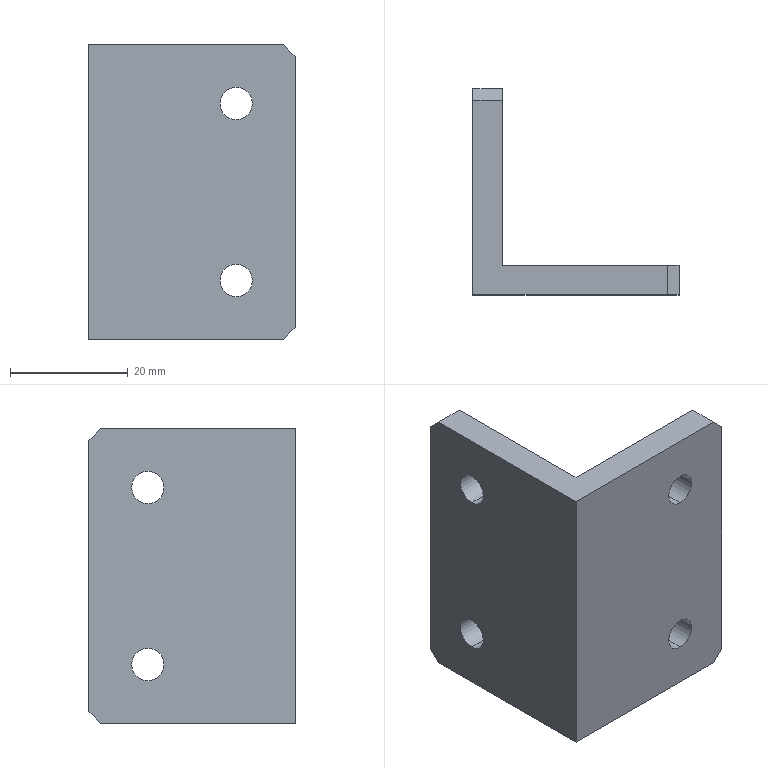Part | STEP file | L bracket | 1 solid | 20 faces | box 35 x 35 x 50 mm | volume 15735 mm3 | plane 12 | cylinder 8 | commonest cylinder face diameters 5.5 x8